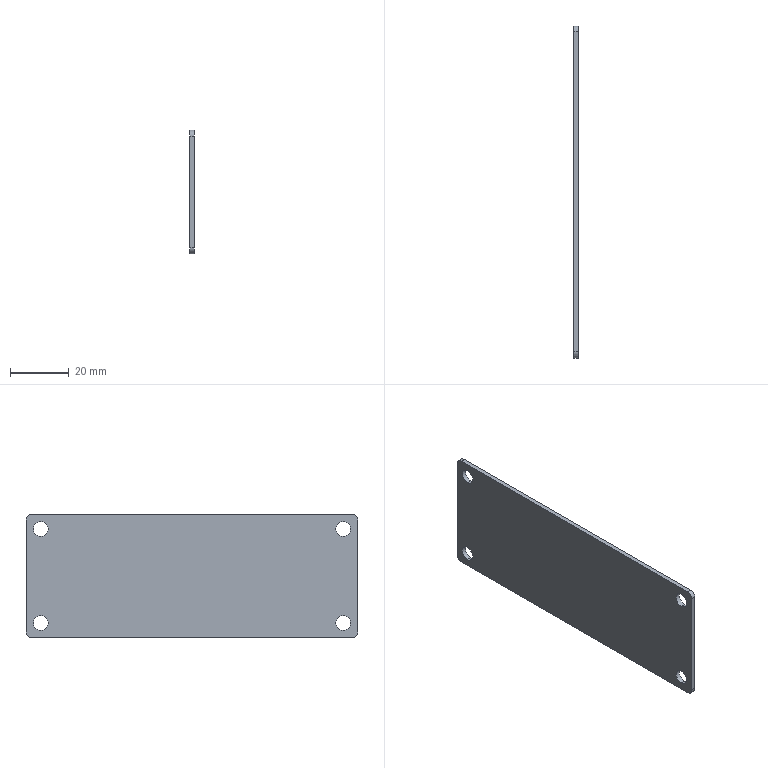Part | NX | features solid 2 | 1 solid | 18 faces | box 1.5 x 113 x 42 mm | volume 6996 mm3 | cylinder 12 | plane 6 | commonest cylinder face diameters 5 x8 4 x4
STEP:
#1=CARTESIAN_POINT('',(-326.5,455.,35.));
#2=VERTEX_POINT('',#1);
#3=CARTESIAN_POINT('',(-326.5,453.,37.));
#4=VERTEX_POINT('',#3);
#5=CARTESIAN_POINT('',(-326.5,453.,35.));
#6=DIRECTION('',(1.,0.,0.));
#7=DIRECTION('',(0.,0.,1.));
#8=AXIS2_PLACEMENT_3D('',#5,#6,#7);
#9=CIRCLE('',#8,2.);
#10=EDGE_CURVE('',#2,#4,#9,.T.);
#11=ORIENTED_EDGE('',*,*,#10,.F.);
#12=CARTESIAN_POINT('',(-328.,455.,35.));
#13=VERTEX_POINT('',#12);
#14=CARTESIAN_POINT('',(-326.5,455.,35.));
#15=DIRECTION('',(1.,0.,0.));
#16=VECTOR('',#15,1000.);
#17=LINE('',#14,#16);
#18=EDGE_CURVE('',#13,#2,#17,.T.);
#19=ORIENTED_EDGE('',*,*,#18,.F.);
#20=CARTESIAN_POINT('',(-328.,453.,37.));
#21=VERTEX_POINT('',#20);
#22=CARTESIAN_POINT('',(-328.,453.,35.));
#23=DIRECTION('',(-1.,0.,0.));
#24=DIRECTION('',(0.,0.,1.));
#25=AXIS2_PLACEMENT_3D('',#22,#23,#24);
#26=CIRCLE('',#25,2.);
#27=EDGE_CURVE('',#21,#13,#26,.T.);
#28=ORIENTED_EDGE('',*,*,#27,.F.);
#29=CARTESIAN_POINT('',(-326.5,453.,37.));
#30=DIRECTION('',(-1.,0.,0.));
#31=VECTOR('',#30,1000.);
#32=LINE('',#29,#31);
#33=EDGE_CURVE('',#4,#21,#32,.T.);
#34=ORIENTED_EDGE('',*,*,#33,.F.);
#35=EDGE_LOOP('',(#11,#19,#28,#34));
#36=FACE_BOUND('',#35,.T.);
#37=CARTESIAN_POINT('',(-326.5,453.,35.));
#38=DIRECTION('',(-1.,0.,0.));
#39=DIRECTION('',(0.,0.,-1.));
#40=AXIS2_PLACEMENT_3D('',#37,#38,#39);
#41=CYLINDRICAL_SURFACE('',#40,2.);
#42=ADVANCED_FACE('',(#36),#41,.T.);
#43=CARTESIAN_POINT('',(-326.5,344.,37.));
#44=VERTEX_POINT('',#43);
#45=CARTESIAN_POINT('',(-326.5,342.,35.));
#46=VERTEX_POINT('',#45);
#47=CARTESIAN_POINT('',(-326.5,344.,35.));
#48=DIRECTION('',(1.,0.,0.));
#49=DIRECTION('',(0.,0.,1.));
#50=AXIS2_PLACEMENT_3D('',#47,#48,#49);
#51=CIRCLE('',#50,2.);
#52=EDGE_CURVE('',#44,#46,#51,.T.);
#53=ORIENTED_EDGE('',*,*,#52,.F.);
#54=CARTESIAN_POINT('',(-328.,344.,37.));
#55=VERTEX_POINT('',#54);
#56=CARTESIAN_POINT('',(-326.5,344.,37.));
#57=DIRECTION('',(1.,0.,0.));
#58=VECTOR('',#57,1000.);
#59=LINE('',#56,#58);
#60=EDGE_CURVE('',#55,#44,#59,.T.);
#61=ORIENTED_EDGE('',*,*,#60,.F.);
#62=CARTESIAN_POINT('',(-328.,342.,35.));
#63=VERTEX_POINT('',#62);
#64=CARTESIAN_POINT('',(-328.,344.,35.));
#65=DIRECTION('',(-1.,0.,0.));
#66=DIRECTION('',(0.,0.,1.));
#67=AXIS2_PLACEMENT_3D('',#64,#65,#66);
#68=CIRCLE('',#67,2.);
#69=EDGE_CURVE('',#63,#55,#68,.T.);
#70=ORIENTED_EDGE('',*,*,#69,.F.);
#71=CARTESIAN_POINT('',(-326.5,342.,35.));
#72=DIRECTION('',(-1.,0.,0.));
#73=VECTOR('',#72,1000.);
#74=LINE('',#71,#73);
#75=EDGE_CURVE('',#46,#63,#74,.T.);
#76=ORIENTED_EDGE('',*,*,#75,.F.);
#77=EDGE_LOOP('',(#53,#61,#70,#76));
#78=FACE_BOUND('',#77,.T.);
#79=CARTESIAN_POINT('',(-326.5,344.,35.));
#80=DIRECTION('',(-1.,0.,0.));
#81=DIRECTION('',(0.,0.,-1.));
#82=AXIS2_PLACEMENT_3D('',#79,#80,#81);
#83=CYLINDRICAL_SURFACE('',#82,2.);
#84=ADVANCED_FACE('',(#78),#83,.T.);
#85=CARTESIAN_POINT('',(-326.5,453.,-5.));
#86=VERTEX_POINT('',#85);
#87=CARTESIAN_POINT('',(-326.5,455.,-3.));
#88=VERTEX_POINT('',#87);
#89=CARTESIAN_POINT('',(-326.5,453.,-3.));
#90=DIRECTION('',(1.,0.,0.));
#91=DIRECTION('',(0.,0.,1.));
#92=AXIS2_PLACEMENT_3D('',#89,#90,#91);
#93=CIRCLE('',#92,2.);
#94=EDGE_CURVE('',#86,#88,#93,.T.);
#95=ORIENTED_EDGE('',*,*,#94,.F.);
#96=CARTESIAN_POINT('',(-328.,453.,-5.));
#97=VERTEX_POINT('',#96);
#98=CARTESIAN_POINT('',(-326.5,453.,-5.));
#99=DIRECTION('',(1.,0.,0.));
#100=VECTOR('',#99,1000.);
#101=LINE('',#98,#100);
#102=EDGE_CURVE('',#97,#86,#101,.T.);
#103=ORIENTED_EDGE('',*,*,#102,.F.);
#104=CARTESIAN_POINT('',(-328.,455.,-3.));
#105=VERTEX_POINT('',#104);
#106=CARTESIAN_POINT('',(-328.,453.,-3.));
#107=DIRECTION('',(-1.,0.,0.));
#108=DIRECTION('',(0.,0.,1.));
#109=AXIS2_PLACEMENT_3D('',#106,#107,#108);
#110=CIRCLE('',#109,2.);
#111=EDGE_CURVE('',#105,#97,#110,.T.);
#112=ORIENTED_EDGE('',*,*,#111,.F.);
#113=CARTESIAN_POINT('',(-326.5,455.,-3.));
#114=DIRECTION('',(-1.,0.,0.));
#115=VECTOR('',#114,1000.);
#116=LINE('',#113,#115);
#117=EDGE_CURVE('',#88,#105,#116,.T.);
#118=ORIENTED_EDGE('',*,*,#117,.F.);
#119=EDGE_LOOP('',(#95,#103,#112,#118));
#120=FACE_BOUND('',#119,.T.);
#121=CARTESIAN_POINT('',(-326.5,453.,-3.));
#122=DIRECTION('',(-1.,0.,0.));
#123=DIRECTION('',(0.,0.,-1.));
#124=AXIS2_PLACEMENT_3D('',#121,#122,#123);
#125=CYLINDRICAL_SURFACE('',#124,2.);
#126=ADVANCED_FACE('',(#120),#125,.T.);
#127=CARTESIAN_POINT('',(-326.5,342.,-3.));
#128=VERTEX_POINT('',#127);
#129=CARTESIAN_POINT('',(-326.5,344.,-5.));
#130=VERTEX_POINT('',#129);
#131=CARTESIAN_POINT('',(-326.5,344.,-3.));
#132=DIRECTION('',(1.,0.,0.));
#133=DIRECTION('',(0.,0.,1.));
#134=AXIS2_PLACEMENT_3D('',#131,#132,#133);
#135=CIRCLE('',#134,2.);
#136=EDGE_CURVE('',#128,#130,#135,.T.);
#137=ORIENTED_EDGE('',*,*,#136,.F.);
#138=CARTESIAN_POINT('',(-328.,342.,-3.));
#139=VERTEX_POINT('',#138);
#140=CARTESIAN_POINT('',(-326.5,342.,-3.));
#141=DIRECTION('',(1.,0.,0.));
#142=VECTOR('',#141,1000.);
#143=LINE('',#140,#142);
#144=EDGE_CURVE('',#139,#128,#143,.T.);
#145=ORIENTED_EDGE('',*,*,#144,.F.);
#146=CARTESIAN_POINT('',(-328.,344.,-5.));
#147=VERTEX_POINT('',#146);
#148=CARTESIAN_POINT('',(-328.,344.,-3.));
#149=DIRECTION('',(-1.,0.,0.));
#150=DIRECTION('',(0.,0.,1.));
#151=AXIS2_PLACEMENT_3D('',#148,#149,#150);
#152=CIRCLE('',#151,2.);
#153=EDGE_CURVE('',#147,#139,#152,.T.);
#154=ORIENTED_EDGE('',*,*,#153,.F.);
#155=CARTESIAN_POINT('',(-326.5,344.,-5.));
#156=DIRECTION('',(-1.,0.,0.));
#157=VECTOR('',#156,1000.);
#158=LINE('',#155,#157);
#159=EDGE_CURVE('',#130,#147,#158,.T.);
#160=ORIENTED_EDGE('',*,*,#159,.F.);
#161=EDGE_LOOP('',(#137,#145,#154,#160));
#162=FACE_BOUND('',#161,.T.);
#163=CARTESIAN_POINT('',(-326.5,344.,-3.));
#164=DIRECTION('',(-1.,0.,0.));
#165=DIRECTION('',(0.,0.,-1.));
#166=AXIS2_PLACEMENT_3D('',#163,#164,#165);
#167=CYLINDRICAL_SURFACE('',#166,2.);
#168=ADVANCED_FACE('',(#162),#167,.T.);
#169=CARTESIAN_POINT('',(-328.,450.,2.5));
#170=VERTEX_POINT('',#169);
#171=CARTESIAN_POINT('',(-326.5,450.,2.5));
#172=VERTEX_POINT('',#171);
#173=CARTESIAN_POINT('',(-207.438,450.,2.5));
#174=DIRECTION('',(-1.,0.,0.));
#175=VECTOR('',#174,1000.);
#176=LINE('',#173,#175);
#177=EDGE_CURVE('',#170,#172,#176,.F.);
#178=ORIENTED_EDGE('',*,*,#177,.T.);
#179=CARTESIAN_POINT('',(-326.5,450.,-2.5));
#180=VERTEX_POINT('',#179);
#181=CARTESIAN_POINT('',(-326.5,450.,0.));
#182=DIRECTION('',(1.,0.,0.));
#183=DIRECTION('',(0.,0.,1.));
#184=AXIS2_PLACEMENT_3D('',#181,#182,#183);
#185=CIRCLE('',#184,2.5);
#186=EDGE_CURVE('',#172,#180,#185,.T.);
#187=ORIENTED_EDGE('',*,*,#186,.T.);
#188=CARTESIAN_POINT('',(-328.,450.,-2.5));
#189=VERTEX_POINT('',#188);
#190=CARTESIAN_POINT('',(-207.438,450.,-2.5));
#191=DIRECTION('',(-1.,0.,0.));
#192=VECTOR('',#191,1000.);
#193=LINE('',#190,#192);
#194=EDGE_CURVE('',#180,#189,#193,.T.);
#195=ORIENTED_EDGE('',*,*,#194,.T.);
#196=CARTESIAN_POINT('',(-328.,450.,0.));
#197=DIRECTION('',(-1.,0.,0.));
#198=DIRECTION('',(0.,-1.,0.));
#199=AXIS2_PLACEMENT_3D('',#196,#197,#198);
#200=CIRCLE('',#199,2.5);
#201=EDGE_CURVE('',#189,#170,#200,.T.);
#202=ORIENTED_EDGE('',*,*,#201,.T.);
#203=EDGE_LOOP('',(#178,#187,#195,#202));
#204=FACE_BOUND('',#203,.T.);
#205=CARTESIAN_POINT('',(-207.438,450.,0.));
#206=DIRECTION('',(-1.,0.,0.));
#207=DIRECTION('',(0.,0.,-1.));
#208=AXIS2_PLACEMENT_3D('',#205,#206,#207);
#209=CYLINDRICAL_SURFACE('',#208,2.5);
#210=ADVANCED_FACE('',(#204),#209,.F.);
#211=CARTESIAN_POINT('',(-328.,347.,2.5));
#212=VERTEX_POINT('',#211);
#213=CARTESIAN_POINT('',(-326.5,347.,2.5));
#214=VERTEX_POINT('',#213);
#215=CARTESIAN_POINT('',(-207.438,347.,2.5));
#216=DIRECTION('',(-1.,0.,0.));
#217=VECTOR('',#216,1000.);
#218=LINE('',#215,#217);
#219=EDGE_CURVE('',#212,#214,#218,.F.);
#220=ORIENTED_EDGE('',*,*,#219,.T.);
#221=CARTESIAN_POINT('',(-326.5,347.,-2.5));
#222=VERTEX_POINT('',#221);
#223=CARTESIAN_POINT('',(-326.5,347.,0.));
#224=DIRECTION('',(1.,0.,0.));
#225=DIRECTION('',(0.,0.,1.));
#226=AXIS2_PLACEMENT_3D('',#223,#224,#225);
#227=CIRCLE('',#226,2.5);
#228=EDGE_CURVE('',#214,#222,#227,.T.);
#229=ORIENTED_EDGE('',*,*,#228,.T.);
#230=CARTESIAN_POINT('',(-328.,347.,-2.5));
#231=VERTEX_POINT('',#230);
#232=CARTESIAN_POINT('',(-207.438,347.,-2.5));
#233=DIRECTION('',(-1.,0.,0.));
#234=VECTOR('',#233,1000.);
#235=LINE('',#232,#234);
#236=EDGE_CURVE('',#222,#231,#235,.T.);
#237=ORIENTED_EDGE('',*,*,#236,.T.);
#238=CARTESIAN_POINT('',(-328.,347.,0.));
#239=DIRECTION('',(-1.,0.,0.));
#240=DIRECTION('',(0.,-1.,0.));
#241=AXIS2_PLACEMENT_3D('',#238,#239,#240);
#242=CIRCLE('',#241,2.5);
#243=EDGE_CURVE('',#231,#212,#242,.T.);
#244=ORIENTED_EDGE('',*,*,#243,.T.);
#245=EDGE_LOOP('',(#220,#229,#237,#244));
#246=FACE_BOUND('',#245,.T.);
#247=CARTESIAN_POINT('',(-207.438,347.,0.));
#248=DIRECTION('',(-1.,0.,0.));
#249=DIRECTION('',(0.,0.,-1.));
#250=AXIS2_PLACEMENT_3D('',#247,#248,#249);
#251=CYLINDRICAL_SURFACE('',#250,2.5);
#252=ADVANCED_FACE('',(#246),#251,.F.);
#253=CARTESIAN_POINT('',(-328.,347.,34.5));
#254=VERTEX_POINT('',#253);
#255=CARTESIAN_POINT('',(-326.5,347.,34.5));
#256=VERTEX_POINT('',#255);
#257=CARTESIAN_POINT('',(-207.438,347.,34.5));
#258=DIRECTION('',(-1.,0.,0.));
#259=VECTOR('',#258,1000.);
#260=LINE('',#257,#259);
#261=EDGE_CURVE('',#254,#256,#260,.F.);
#262=ORIENTED_EDGE('',*,*,#261,.T.);
#263=CARTESIAN_POINT('',(-326.5,347.,29.5));
#264=VERTEX_POINT('',#263);
#265=CARTESIAN_POINT('',(-326.5,347.,32.));
#266=DIRECTION('',(1.,0.,0.));
#267=DIRECTION('',(0.,0.,1.));
#268=AXIS2_PLACEMENT_3D('',#265,#266,#267);
#269=CIRCLE('',#268,2.5);
#270=EDGE_CURVE('',#256,#264,#269,.T.);
#271=ORIENTED_EDGE('',*,*,#270,.T.);
#272=CARTESIAN_POINT('',(-328.,347.,29.5));
#273=VERTEX_POINT('',#272);
#274=CARTESIAN_POINT('',(-207.438,347.,29.5));
#275=DIRECTION('',(-1.,0.,0.));
#276=VECTOR('',#275,1000.);
#277=LINE('',#274,#276);
#278=EDGE_CURVE('',#264,#273,#277,.T.);
#279=ORIENTED_EDGE('',*,*,#278,.T.);
#280=CARTESIAN_POINT('',(-328.,347.,32.));
#281=DIRECTION('',(-1.,0.,0.));
#282=DIRECTION('',(0.,-1.,0.));
#283=AXIS2_PLACEMENT_3D('',#280,#281,#282);
#284=CIRCLE('',#283,2.5);
#285=EDGE_CURVE('',#273,#254,#284,.T.);
#286=ORIENTED_EDGE('',*,*,#285,.T.);
#287=EDGE_LOOP('',(#262,#271,#279,#286));
#288=FACE_BOUND('',#287,.T.);
#289=CARTESIAN_POINT('',(-207.438,347.,32.));
#290=DIRECTION('',(-1.,0.,0.));
#291=DIRECTION('',(0.,0.,-1.));
#292=AXIS2_PLACEMENT_3D('',#289,#290,#291);
#293=CYLINDRICAL_SURFACE('',#292,2.5);
#294=ADVANCED_FACE('',(#288),#293,.F.);
#295=CARTESIAN_POINT('',(-328.,450.,34.5));
#296=VERTEX_POINT('',#295);
#297=CARTESIAN_POINT('',(-326.5,450.,34.5));
#298=VERTEX_POINT('',#297);
#299=CARTESIAN_POINT('',(-207.438,450.,34.5));
#300=DIRECTION('',(-1.,0.,0.));
#301=VECTOR('',#300,1000.);
#302=LINE('',#299,#301);
#303=EDGE_CURVE('',#296,#298,#302,.F.);
#304=ORIENTED_EDGE('',*,*,#303,.T.);
#305=CARTESIAN_POINT('',(-326.5,450.,29.5));
#306=VERTEX_POINT('',#305);
#307=CARTESIAN_POINT('',(-326.5,450.,32.));
#308=DIRECTION('',(1.,0.,0.));
#309=DIRECTION('',(0.,0.,1.));
#310=AXIS2_PLACEMENT_3D('',#307,#308,#309);
#311=CIRCLE('',#310,2.5);
#312=EDGE_CURVE('',#298,#306,#311,.T.);
#313=ORIENTED_EDGE('',*,*,#312,.T.);
#314=CARTESIAN_POINT('',(-328.,450.,29.5));
#315=VERTEX_POINT('',#314);
#316=CARTESIAN_POINT('',(-207.438,450.,29.5));
#317=DIRECTION('',(-1.,0.,0.));
#318=VECTOR('',#317,1000.);
#319=LINE('',#316,#318);
#320=EDGE_CURVE('',#306,#315,#319,.T.);
#321=ORIENTED_EDGE('',*,*,#320,.T.);
#322=CARTESIAN_POINT('',(-328.,450.,32.));
#323=DIRECTION('',(-1.,0.,0.));
#324=DIRECTION('',(0.,-1.,0.));
#325=AXIS2_PLACEMENT_3D('',#322,#323,#324);
#326=CIRCLE('',#325,2.5);
#327=EDGE_CURVE('',#315,#296,#326,.T.);
#328=ORIENTED_EDGE('',*,*,#327,.T.);
#329=EDGE_LOOP('',(#304,#313,#321,#328));
#330=FACE_BOUND('',#329,.T.);
#331=CARTESIAN_POINT('',(-207.438,450.,32.));
#332=DIRECTION('',(-1.,0.,0.));
#333=DIRECTION('',(0.,0.,-1.));
#334=AXIS2_PLACEMENT_3D('',#331,#332,#333);
#335=CYLINDRICAL_SURFACE('',#334,2.5);
#336=ADVANCED_FACE('',(#330),#335,.F.);
#337=ORIENTED_EDGE('',*,*,#327,.F.);
#338=CARTESIAN_POINT('',(-328.,450.,32.));
#339=DIRECTION('',(-1.,0.,0.));
#340=DIRECTION('',(0.,-1.,0.));
#341=AXIS2_PLACEMENT_3D('',#338,#339,#340);
#342=CIRCLE('',#341,2.5);
#343=EDGE_CURVE('',#296,#315,#342,.T.);
#344=ORIENTED_EDGE('',*,*,#343,.F.);
#345=EDGE_LOOP('',(#337,#344));
#346=FACE_BOUND('',#345,.T.);
#347=ORIENTED_EDGE('',*,*,#285,.F.);
#348=CARTESIAN_POINT('',(-328.,347.,32.));
#349=DIRECTION('',(-1.,0.,0.));
#350=DIRECTION('',(0.,-1.,0.));
#351=AXIS2_PLACEMENT_3D('',#348,#349,#350);
#352=CIRCLE('',#351,2.5);
#353=EDGE_CURVE('',#254,#273,#352,.T.);
#354=ORIENTED_EDGE('',*,*,#353,.F.);
#355=EDGE_LOOP('',(#347,#354));
#356=FACE_BOUND('',#355,.T.);
#357=ORIENTED_EDGE('',*,*,#243,.F.);
#358=CARTESIAN_POINT('',(-328.,347.,0.));
#359=DIRECTION('',(-1.,0.,0.));
#360=DIRECTION('',(0.,-1.,0.));
#361=AXIS2_PLACEMENT_3D('',#358,#359,#360);
#362=CIRCLE('',#361,2.5);
#363=EDGE_CURVE('',#212,#231,#362,.T.);
#364=ORIENTED_EDGE('',*,*,#363,.F.);
#365=EDGE_LOOP('',(#357,#364));
#366=FACE_BOUND('',#365,.T.);
#367=ORIENTED_EDGE('',*,*,#201,.F.);
#368=CARTESIAN_POINT('',(-328.,450.,0.));
#369=DIRECTION('',(-1.,0.,0.));
#370=DIRECTION('',(0.,-1.,0.));
#371=AXIS2_PLACEMENT_3D('',#368,#369,#370);
#372=CIRCLE('',#371,2.5);
#373=EDGE_CURVE('',#170,#189,#372,.T.);
#374=ORIENTED_EDGE('',*,*,#373,.F.);
#375=EDGE_LOOP('',(#367,#374));
#376=FACE_BOUND('',#375,.T.);
#377=CARTESIAN_POINT('',(-328.,342.,-5.));
#378=DIRECTION('',(0.,1.,0.));
#379=VECTOR('',#378,1000.);
#380=LINE('',#377,#379);
#381=EDGE_CURVE('',#147,#97,#380,.T.);
#382=ORIENTED_EDGE('',*,*,#381,.F.);
#383=ORIENTED_EDGE('',*,*,#153,.T.);
#384=CARTESIAN_POINT('',(-328.,342.,37.));
#385=DIRECTION('',(0.,0.,-1.));
#386=VECTOR('',#385,1000.);
#387=LINE('',#384,#386);
#388=EDGE_CURVE('',#63,#139,#387,.T.);
#389=ORIENTED_EDGE('',*,*,#388,.F.);
#390=ORIENTED_EDGE('',*,*,#69,.T.);
#391=CARTESIAN_POINT('',(-328.,455.,37.));
#392=DIRECTION('',(0.,-1.,0.));
#393=VECTOR('',#392,1000.);
#394=LINE('',#391,#393);
#395=EDGE_CURVE('',#21,#55,#394,.T.);
#396=ORIENTED_EDGE('',*,*,#395,.F.);
#397=ORIENTED_EDGE('',*,*,#27,.T.);
#398=CARTESIAN_POINT('',(-328.,455.,-5.));
#399=DIRECTION('',(0.,0.,1.));
#400=VECTOR('',#399,1000.);
#401=LINE('',#398,#400);
#402=EDGE_CURVE('',#105,#13,#401,.T.);
#403=ORIENTED_EDGE('',*,*,#402,.F.);
#404=ORIENTED_EDGE('',*,*,#111,.T.);
#405=EDGE_LOOP('',(#382,#383,#389,#390,#396,#397,#403,#404));
#406=FACE_BOUND('',#405,.T.);
#407=CARTESIAN_POINT('',(-328.,398.5,16.));
#408=DIRECTION('',(1.,0.,0.));
#409=DIRECTION('',(0.,0.,1.));
#410=AXIS2_PLACEMENT_3D('',#407,#408,#409);
#411=PLANE('',#410);
#412=ADVANCED_FACE('',(#346,#356,#366,#376,#406),#411,.F.);
#413=CARTESIAN_POINT('',(-326.5,450.,32.));
#414=DIRECTION('',(1.,0.,0.));
#415=DIRECTION('',(0.,0.,1.));
#416=AXIS2_PLACEMENT_3D('',#413,#414,#415);
#417=CIRCLE('',#416,2.5);
#418=EDGE_CURVE('',#306,#298,#417,.T.);
#419=ORIENTED_EDGE('',*,*,#418,.F.);
#420=ORIENTED_EDGE('',*,*,#312,.F.);
#421=EDGE_LOOP('',(#419,#420));
#422=FACE_BOUND('',#421,.T.);
#423=CARTESIAN_POINT('',(-326.5,347.,32.));
#424=DIRECTION('',(1.,0.,0.));
#425=DIRECTION('',(0.,0.,1.));
#426=AXIS2_PLACEMENT_3D('',#423,#424,#425);
#427=CIRCLE('',#426,2.5);
#428=EDGE_CURVE('',#264,#256,#427,.T.);
#429=ORIENTED_EDGE('',*,*,#428,.F.);
#430=ORIENTED_EDGE('',*,*,#270,.F.);
#431=EDGE_LOOP('',(#429,#430));
#432=FACE_BOUND('',#431,.T.);
#433=CARTESIAN_POINT('',(-326.5,347.,0.));
#434=DIRECTION('',(1.,0.,0.));
#435=DIRECTION('',(0.,0.,1.));
#436=AXIS2_PLACEMENT_3D('',#433,#434,#435);
#437=CIRCLE('',#436,2.5);
#438=EDGE_CURVE('',#222,#214,#437,.T.);
#439=ORIENTED_EDGE('',*,*,#438,.F.);
#440=ORIENTED_EDGE('',*,*,#228,.F.);
#441=EDGE_LOOP('',(#439,#440));
#442=FACE_BOUND('',#441,.T.);
#443=CARTESIAN_POINT('',(-326.5,450.,0.));
#444=DIRECTION('',(1.,0.,0.));
#445=DIRECTION('',(0.,0.,1.));
#446=AXIS2_PLACEMENT_3D('',#443,#444,#445);
#447=CIRCLE('',#446,2.5);
#448=EDGE_CURVE('',#180,#172,#447,.T.);
#449=ORIENTED_EDGE('',*,*,#448,.F.);
#450=ORIENTED_EDGE('',*,*,#186,.F.);
#451=EDGE_LOOP('',(#449,#450));
#452=FACE_BOUND('',#451,.T.);
#453=CARTESIAN_POINT('',(-326.5,342.,37.));
#454=DIRECTION('',(0.,0.,-1.));
#455=VECTOR('',#454,1000.);
#456=LINE('',#453,#455);
#457=EDGE_CURVE('',#46,#128,#456,.T.);
#458=ORIENTED_EDGE('',*,*,#457,.T.);
#459=ORIENTED_EDGE('',*,*,#136,.T.);
#460=CARTESIAN_POINT('',(-326.5,342.,-5.));
#461=DIRECTION('',(0.,1.,0.));
#462=VECTOR('',#461,1000.);
#463=LINE('',#460,#462);
#464=EDGE_CURVE('',#130,#86,#463,.T.);
#465=ORIENTED_EDGE('',*,*,#464,.T.);
#466=ORIENTED_EDGE('',*,*,#94,.T.);
#467=CARTESIAN_POINT('',(-326.5,455.,-5.));
#468=DIRECTION('',(0.,0.,1.));
#469=VECTOR('',#468,1000.);
#470=LINE('',#467,#469);
#471=EDGE_CURVE('',#88,#2,#470,.T.);
#472=ORIENTED_EDGE('',*,*,#471,.T.);
#473=ORIENTED_EDGE('',*,*,#10,.T.);
#474=CARTESIAN_POINT('',(-326.5,455.,37.));
#475=DIRECTION('',(0.,-1.,0.));
#476=VECTOR('',#475,1000.);
#477=LINE('',#474,#476);
#478=EDGE_CURVE('',#4,#44,#477,.T.);
#479=ORIENTED_EDGE('',*,*,#478,.T.);
#480=ORIENTED_EDGE('',*,*,#52,.T.);
#481=EDGE_LOOP('',(#458,#459,#465,#466,#472,#473,#479,#480));
#482=FACE_BOUND('',#481,.T.);
#483=CARTESIAN_POINT('',(-326.5,398.5,16.));
#484=DIRECTION('',(1.,0.,0.));
#485=DIRECTION('',(0.,0.,1.));
#486=AXIS2_PLACEMENT_3D('',#483,#484,#485);
#487=PLANE('',#486);
#488=ADVANCED_FACE('',(#422,#432,#442,#452,#482),#487,.T.);
#489=ORIENTED_EDGE('',*,*,#395,.T.);
#490=ORIENTED_EDGE('',*,*,#60,.T.);
#491=ORIENTED_EDGE('',*,*,#478,.F.);
#492=ORIENTED_EDGE('',*,*,#33,.T.);
#493=EDGE_LOOP('',(#489,#490,#491,#492));
#494=FACE_BOUND('',#493,.T.);
#495=CARTESIAN_POINT('',(-326.5,455.,37.));
#496=DIRECTION('',(0.,0.,-1.));
#497=DIRECTION('',(0.,-1.,0.));
#498=AXIS2_PLACEMENT_3D('',#495,#496,#497);
#499=PLANE('',#498);
#500=ADVANCED_FACE('',(#494),#499,.F.);
#501=ORIENTED_EDGE('',*,*,#471,.F.);
#502=ORIENTED_EDGE('',*,*,#117,.T.);
#503=ORIENTED_EDGE('',*,*,#402,.T.);
#504=ORIENTED_EDGE('',*,*,#18,.T.);
#505=EDGE_LOOP('',(#501,#502,#503,#504));
#506=FACE_BOUND('',#505,.T.);
#507=CARTESIAN_POINT('',(-326.5,455.,-5.));
#508=DIRECTION('',(0.,-1.,0.));
#509=DIRECTION('',(-1.,0.,0.));
#510=AXIS2_PLACEMENT_3D('',#507,#508,#509);
#511=PLANE('',#510);
#512=ADVANCED_FACE('',(#506),#511,.F.);
#513=ORIENTED_EDGE('',*,*,#464,.F.);
#514=ORIENTED_EDGE('',*,*,#159,.T.);
#515=ORIENTED_EDGE('',*,*,#381,.T.);
#516=ORIENTED_EDGE('',*,*,#102,.T.);
#517=EDGE_LOOP('',(#513,#514,#515,#516));
#518=FACE_BOUND('',#517,.T.);
#519=CARTESIAN_POINT('',(-326.5,342.,-5.));
#520=DIRECTION('',(0.,0.,1.));
#521=DIRECTION('',(0.,-1.,0.));
#522=AXIS2_PLACEMENT_3D('',#519,#520,#521);
#523=PLANE('',#522);
#524=ADVANCED_FACE('',(#518),#523,.F.);
#525=ORIENTED_EDGE('',*,*,#388,.T.);
#526=ORIENTED_EDGE('',*,*,#144,.T.);
#527=ORIENTED_EDGE('',*,*,#457,.F.);
#528=ORIENTED_EDGE('',*,*,#75,.T.);
#529=EDGE_LOOP('',(#525,#526,#527,#528));
#530=FACE_BOUND('',#529,.T.);
#531=CARTESIAN_POINT('',(-326.5,342.,37.));
#532=DIRECTION('',(0.,1.,0.));
#533=DIRECTION('',(0.,0.,-1.));
#534=AXIS2_PLACEMENT_3D('',#531,#532,#533);
#535=PLANE('',#534);
#536=ADVANCED_FACE('',(#530),#535,.F.);
#537=ORIENTED_EDGE('',*,*,#418,.T.);
#538=ORIENTED_EDGE('',*,*,#303,.F.);
#539=ORIENTED_EDGE('',*,*,#343,.T.);
#540=ORIENTED_EDGE('',*,*,#320,.F.);
#541=EDGE_LOOP('',(#537,#538,#539,#540));
#542=FACE_BOUND('',#541,.T.);
#543=CARTESIAN_POINT('',(-207.438,450.,32.));
#544=DIRECTION('',(-1.,0.,0.));
#545=DIRECTION('',(0.,0.,-1.));
#546=AXIS2_PLACEMENT_3D('',#543,#544,#545);
#547=CYLINDRICAL_SURFACE('',#546,2.5);
#548=ADVANCED_FACE('',(#542),#547,.F.);
#549=ORIENTED_EDGE('',*,*,#428,.T.);
#550=ORIENTED_EDGE('',*,*,#261,.F.);
#551=ORIENTED_EDGE('',*,*,#353,.T.);
#552=ORIENTED_EDGE('',*,*,#278,.F.);
#553=EDGE_LOOP('',(#549,#550,#551,#552));
#554=FACE_BOUND('',#553,.T.);
#555=CARTESIAN_POINT('',(-207.438,347.,32.));
#556=DIRECTION('',(-1.,0.,0.));
#557=DIRECTION('',(0.,0.,-1.));
#558=AXIS2_PLACEMENT_3D('',#555,#556,#557);
#559=CYLINDRICAL_SURFACE('',#558,2.5);
#560=ADVANCED_FACE('',(#554),#559,.F.);
#561=ORIENTED_EDGE('',*,*,#438,.T.);
#562=ORIENTED_EDGE('',*,*,#219,.F.);
#563=ORIENTED_EDGE('',*,*,#363,.T.);
#564=ORIENTED_EDGE('',*,*,#236,.F.);
#565=EDGE_LOOP('',(#561,#562,#563,#564));
#566=FACE_BOUND('',#565,.T.);
#567=CARTESIAN_POINT('',(-207.438,347.,0.));
#568=DIRECTION('',(-1.,0.,0.));
#569=DIRECTION('',(0.,0.,-1.));
#570=AXIS2_PLACEMENT_3D('',#567,#568,#569);
#571=CYLINDRICAL_SURFACE('',#570,2.5);
#572=ADVANCED_FACE('',(#566),#571,.F.);
#573=ORIENTED_EDGE('',*,*,#448,.T.);
#574=ORIENTED_EDGE('',*,*,#177,.F.);
#575=ORIENTED_EDGE('',*,*,#373,.T.);
#576=ORIENTED_EDGE('',*,*,#194,.F.);
#577=EDGE_LOOP('',(#573,#574,#575,#576));
#578=FACE_BOUND('',#577,.T.);
#579=CARTESIAN_POINT('',(-207.438,450.,0.));
#580=DIRECTION('',(-1.,0.,0.));
#581=DIRECTION('',(0.,0.,-1.));
#582=AXIS2_PLACEMENT_3D('',#579,#580,#581);
#583=CYLINDRICAL_SURFACE('',#582,2.5);
#584=ADVANCED_FACE('',(#578),#583,.F.);
#585=CLOSED_SHELL('',(#42,#84,#126,#168,#210,#252,#294,#336,#412,#488,#500,#512,#524,#536,#548,#560,#572,#584));
#586=MANIFOLD_SOLID_BREP('',#585);
#587=(LENGTH_UNIT()NAMED_UNIT(*)SI_UNIT(.MILLI.,.METRE.));
#588=UNCERTAINTY_MEASURE_WITH_UNIT(LENGTH_MEASURE(0.00001),#587,'','');
#589=(NAMED_UNIT(*)PLANE_ANGLE_UNIT()SI_UNIT($,.RADIAN.));
#590=(NAMED_UNIT(*)SI_UNIT($,.STERADIAN.)SOLID_ANGLE_UNIT());
#591=(GEOMETRIC_REPRESENTATION_CONTEXT(3)GLOBAL_UNCERTAINTY_ASSIGNED_CONTEXT((#588))GLOBAL_UNIT_ASSIGNED_CONTEXT((#587,#589,#590))REPRESENTATION_CONTEXT('',''));
#592=ADVANCED_BREP_SHAPE_REPRESENTATION('',(#586),#591);